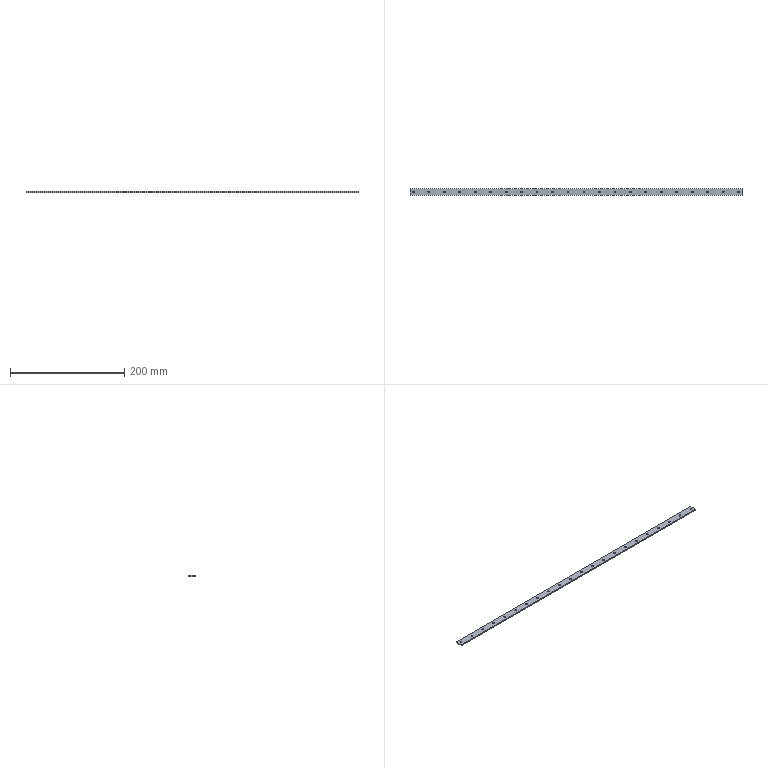Part | SolidWorks | features BaseBody 1 | 1 solid | 50 faces | box 580 x 12 x 2 mm | volume 13566 mm3 | cylinder 44 | plane 6 | commonest cylinder face diameters 3.2 x44